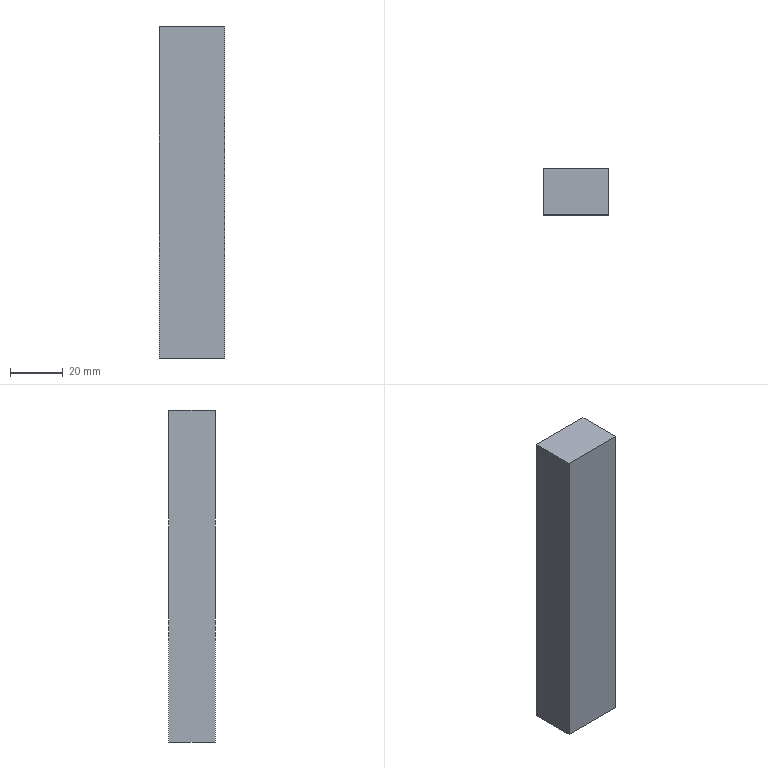Part | SolidWorks | features Extrusion 1 | 1 solid | 6 faces | box 25 x 17.5 x 126 mm | volume 55125 mm3 | plane 6
STEP:
#1=CARTESIAN_POINT('',(-12.5,-8.75,-63.));
#2=VERTEX_POINT('',#1);
#3=CARTESIAN_POINT('',(-12.5,-8.75,63.));
#4=VERTEX_POINT('',#3);
#5=CARTESIAN_POINT('',(-12.5,-8.75,-63.));
#6=DIRECTION('',(0.,0.,1.));
#7=VECTOR('',#6,1000.);
#8=LINE('',#5,#7);
#9=EDGE_CURVE('',#2,#4,#8,.T.);
#10=ORIENTED_EDGE('',*,*,#9,.T.);
#11=CARTESIAN_POINT('',(-12.5,8.75,63.));
#12=VERTEX_POINT('',#11);
#13=CARTESIAN_POINT('',(-12.5,8.75,63.));
#14=DIRECTION('',(0.,-1.,0.));
#15=VECTOR('',#14,1000.);
#16=LINE('',#13,#15);
#17=EDGE_CURVE('',#12,#4,#16,.T.);
#18=ORIENTED_EDGE('',*,*,#17,.F.);
#19=CARTESIAN_POINT('',(-12.5,8.75,-63.));
#20=VERTEX_POINT('',#19);
#21=CARTESIAN_POINT('',(-12.5,8.75,-63.));
#22=DIRECTION('',(0.,0.,1.));
#23=VECTOR('',#22,1000.);
#24=LINE('',#21,#23);
#25=EDGE_CURVE('',#20,#12,#24,.T.);
#26=ORIENTED_EDGE('',*,*,#25,.F.);
#27=CARTESIAN_POINT('',(-12.5,8.75,-63.));
#28=DIRECTION('',(0.,-1.,0.));
#29=VECTOR('',#28,1000.);
#30=LINE('',#27,#29);
#31=EDGE_CURVE('',#20,#2,#30,.T.);
#32=ORIENTED_EDGE('',*,*,#31,.T.);
#33=EDGE_LOOP('',(#10,#18,#26,#32));
#34=FACE_OUTER_BOUND('',#33,.T.);
#35=CARTESIAN_POINT('',(-12.5,8.75,-63.));
#36=DIRECTION('',(1.,0.,0.));
#37=DIRECTION('',(0.,0.,-1.));
#38=AXIS2_PLACEMENT_3D('',#35,#36,#37);
#39=PLANE('',#38);
#40=ADVANCED_FACE('',(#34),#39,.F.);
#41=CARTESIAN_POINT('',(12.5,-8.75,63.));
#42=VERTEX_POINT('',#41);
#43=CARTESIAN_POINT('',(-12.5,-8.75,63.));
#44=DIRECTION('',(1.,0.,0.));
#45=VECTOR('',#44,1000.);
#46=LINE('',#43,#45);
#47=EDGE_CURVE('',#4,#42,#46,.T.);
#48=ORIENTED_EDGE('',*,*,#47,.T.);
#49=CARTESIAN_POINT('',(12.5,8.75,63.));
#50=VERTEX_POINT('',#49);
#51=CARTESIAN_POINT('',(12.5,8.75,63.));
#52=DIRECTION('',(0.,-1.,0.));
#53=VECTOR('',#52,1000.);
#54=LINE('',#51,#53);
#55=EDGE_CURVE('',#50,#42,#54,.T.);
#56=ORIENTED_EDGE('',*,*,#55,.F.);
#57=CARTESIAN_POINT('',(-12.5,8.75,63.));
#58=DIRECTION('',(1.,0.,0.));
#59=VECTOR('',#58,1000.);
#60=LINE('',#57,#59);
#61=EDGE_CURVE('',#12,#50,#60,.T.);
#62=ORIENTED_EDGE('',*,*,#61,.F.);
#63=ORIENTED_EDGE('',*,*,#17,.T.);
#64=EDGE_LOOP('',(#48,#56,#62,#63));
#65=FACE_OUTER_BOUND('',#64,.T.);
#66=CARTESIAN_POINT('',(-12.5,8.75,63.));
#67=DIRECTION('',(0.,0.,-1.));
#68=DIRECTION('',(-1.,0.,0.));
#69=AXIS2_PLACEMENT_3D('',#66,#67,#68);
#70=PLANE('',#69);
#71=ADVANCED_FACE('',(#65),#70,.F.);
#72=CARTESIAN_POINT('',(12.5,-8.75,-63.));
#73=VERTEX_POINT('',#72);
#74=CARTESIAN_POINT('',(12.5,-8.75,-63.));
#75=DIRECTION('',(0.,0.,-1.));
#76=VECTOR('',#75,1000.);
#77=LINE('',#74,#76);
#78=EDGE_CURVE('',#42,#73,#77,.T.);
#79=ORIENTED_EDGE('',*,*,#78,.T.);
#80=CARTESIAN_POINT('',(12.5,8.75,-63.));
#81=VERTEX_POINT('',#80);
#82=CARTESIAN_POINT('',(12.5,8.75,-63.));
#83=DIRECTION('',(0.,-1.,0.));
#84=VECTOR('',#83,1000.);
#85=LINE('',#82,#84);
#86=EDGE_CURVE('',#81,#73,#85,.T.);
#87=ORIENTED_EDGE('',*,*,#86,.F.);
#88=CARTESIAN_POINT('',(12.5,8.75,-63.));
#89=DIRECTION('',(0.,0.,-1.));
#90=VECTOR('',#89,1000.);
#91=LINE('',#88,#90);
#92=EDGE_CURVE('',#50,#81,#91,.T.);
#93=ORIENTED_EDGE('',*,*,#92,.F.);
#94=ORIENTED_EDGE('',*,*,#55,.T.);
#95=EDGE_LOOP('',(#79,#87,#93,#94));
#96=FACE_OUTER_BOUND('',#95,.T.);
#97=CARTESIAN_POINT('',(12.5,8.75,-63.));
#98=DIRECTION('',(-1.,0.,0.));
#99=DIRECTION('',(0.,0.,1.));
#100=AXIS2_PLACEMENT_3D('',#97,#98,#99);
#101=PLANE('',#100);
#102=ADVANCED_FACE('',(#96),#101,.F.);
#103=CARTESIAN_POINT('',(-12.5,-8.75,-63.));
#104=DIRECTION('',(-1.,0.,0.));
#105=VECTOR('',#104,1000.);
#106=LINE('',#103,#105);
#107=EDGE_CURVE('',#73,#2,#106,.T.);
#108=ORIENTED_EDGE('',*,*,#107,.T.);
#109=ORIENTED_EDGE('',*,*,#31,.F.);
#110=CARTESIAN_POINT('',(-12.5,8.75,-63.));
#111=DIRECTION('',(-1.,0.,0.));
#112=VECTOR('',#111,1000.);
#113=LINE('',#110,#112);
#114=EDGE_CURVE('',#81,#20,#113,.T.);
#115=ORIENTED_EDGE('',*,*,#114,.F.);
#116=ORIENTED_EDGE('',*,*,#86,.T.);
#117=EDGE_LOOP('',(#108,#109,#115,#116));
#118=FACE_OUTER_BOUND('',#117,.T.);
#119=CARTESIAN_POINT('',(-12.5,8.75,-63.));
#120=DIRECTION('',(0.,0.,1.));
#121=DIRECTION('',(1.,0.,0.));
#122=AXIS2_PLACEMENT_3D('',#119,#120,#121);
#123=PLANE('',#122);
#124=ADVANCED_FACE('',(#118),#123,.F.);
#125=ORIENTED_EDGE('',*,*,#25,.T.);
#126=ORIENTED_EDGE('',*,*,#61,.T.);
#127=ORIENTED_EDGE('',*,*,#92,.T.);
#128=ORIENTED_EDGE('',*,*,#114,.T.);
#129=EDGE_LOOP('',(#125,#126,#127,#128));
#130=FACE_OUTER_BOUND('',#129,.T.);
#131=CARTESIAN_POINT('',(0.,8.75,0.));
#132=DIRECTION('',(0.,1.,0.));
#133=DIRECTION('',(0.,0.,1.));
#134=AXIS2_PLACEMENT_3D('',#131,#132,#133);
#135=PLANE('',#134);
#136=ADVANCED_FACE('',(#130),#135,.T.);
#137=ORIENTED_EDGE('',*,*,#9,.F.);
#138=ORIENTED_EDGE('',*,*,#107,.F.);
#139=ORIENTED_EDGE('',*,*,#78,.F.);
#140=ORIENTED_EDGE('',*,*,#47,.F.);
#141=EDGE_LOOP('',(#137,#138,#139,#140));
#142=FACE_OUTER_BOUND('',#141,.T.);
#143=CARTESIAN_POINT('',(0.,-8.75,0.));
#144=DIRECTION('',(0.,1.,0.));
#145=DIRECTION('',(0.,0.,1.));
#146=AXIS2_PLACEMENT_3D('',#143,#144,#145);
#147=PLANE('',#146);
#148=ADVANCED_FACE('',(#142),#147,.F.);
#149=CLOSED_SHELL('',(#40,#71,#102,#124,#136,#148));
#150=MANIFOLD_SOLID_BREP('',#149);
#151=CARTESIAN_POINT('',(0.,0.,0.));
#152=DIRECTION('',(0.,0.,1.));
#153=DIRECTION('',(1.,0.,0.));
#154=AXIS2_PLACEMENT_3D('',#151,#152,#153);
#155=(LENGTH_UNIT()NAMED_UNIT(*)SI_UNIT(.MILLI.,.METRE.));
#156=UNCERTAINTY_MEASURE_WITH_UNIT(LENGTH_MEASURE(0.00001),#155,'','');
#157=(NAMED_UNIT(*)PLANE_ANGLE_UNIT()SI_UNIT($,.RADIAN.));
#158=(NAMED_UNIT(*)SI_UNIT($,.STERADIAN.)SOLID_ANGLE_UNIT());
#159=(GEOMETRIC_REPRESENTATION_CONTEXT(3)GLOBAL_UNCERTAINTY_ASSIGNED_CONTEXT((#156))GLOBAL_UNIT_ASSIGNED_CONTEXT((#155,#157,#158))REPRESENTATION_CONTEXT('',''));
#160=ADVANCED_BREP_SHAPE_REPRESENTATION('',(#150,#154),#159);